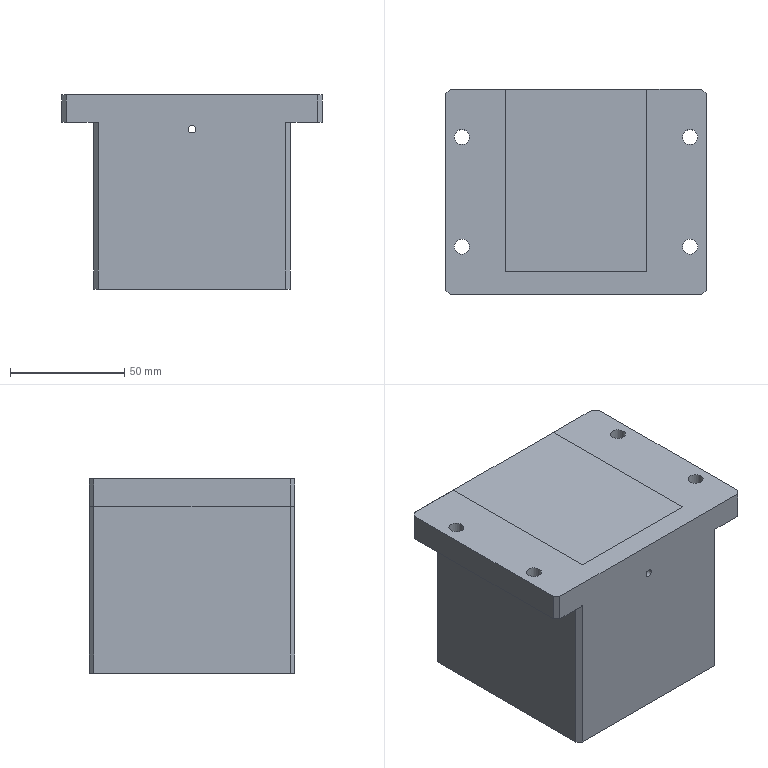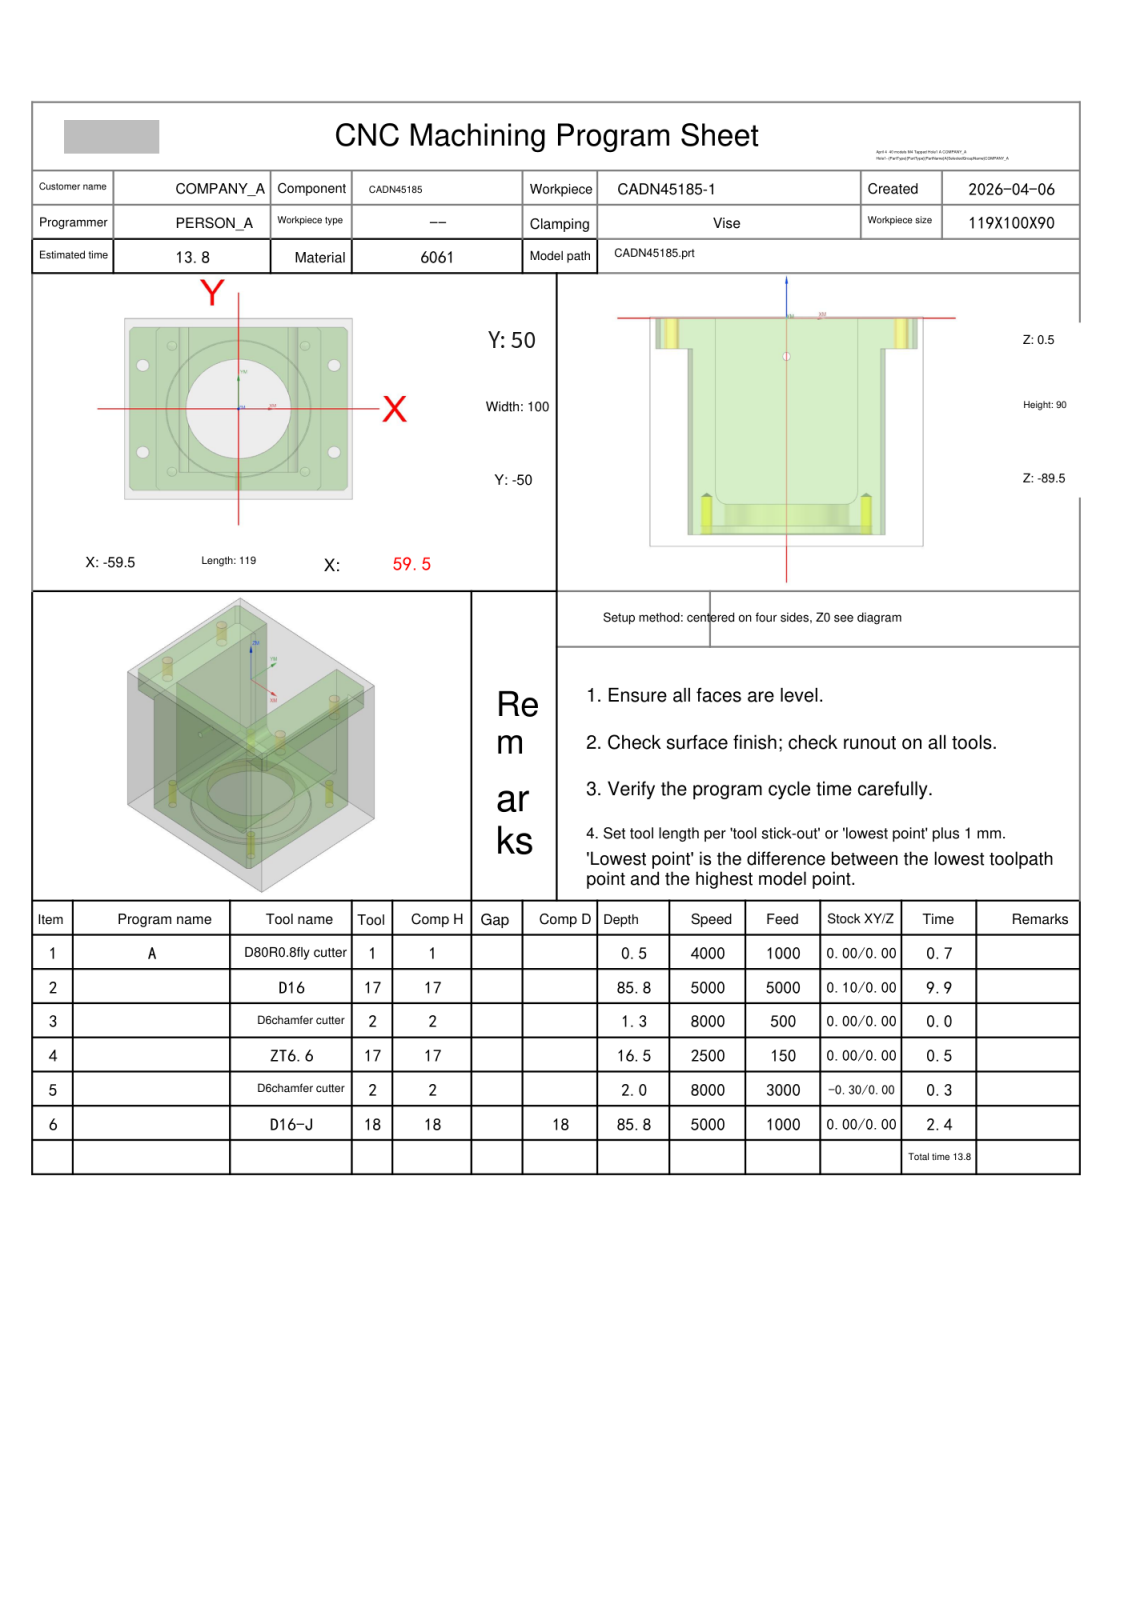NC program | NX | posted by the shop | part box 114 x 90 x 85 mm
Lines 1795 to 2085 of 2085:
N3 T02 M06
(D6chamfer cutter  D=6. R=0. H=02 ce=0.00 di=0.00)
G00 G90 G54 X50. Y-24. M03 S8000
G43 H02 Z20.
M08
G98 G81 X50. Y-24. Z-.8 R1. F500.
Y24.
X-50.
Y-24.
G80
G00 Z20.
G91 G28 Z0.0
M05
M09
G91 G28 Z0.0
M01
N4 T17 M06
(ZT6.6 D=6.6 DR_a=118 H=17)
G00 G90 G54 X50. Y-24. M03 S2500
G43 H17 Z20.
M08
G98 G83 X50. Y-24. Z-15.983 R1. F150. Q3.
Y24.
X-50.
Y-24.
G80
G00 Z20.
G91 G28 Z0.0
M05
M09
G91 G28 Z0.0
M01
N5 T02 M06
(D6chamfer cutter  D=6. R=0. H=02 ce=0.00 di=0.00)
G00 G90 G54 X.25 Y-47.128 M03 S8000
G43 H02 Z20.
M08
Z2.099
G01 Z-1.5 F3000.
G03 X.33 Y-46.828 I-.52 J.3
X.03 Y-46.308 I-.6 J0.0
G01 X0.0 Y-46.3
X-55.
X-55.254 Y-46.275
X-55.497 Y-46.201
X-55.722 Y-46.081
X-55.919 Y-45.919
X-57.919 Y-43.919
X-58.081 Y-43.722
X-58.201 Y-43.497
X-58.275 Y-43.254
X-58.3 Y-43.
Y43.
X-58.275 Y43.254
X-58.201 Y43.497
X-58.081 Y43.722
X-57.919 Y43.919
X-55.919 Y45.919
X-55.722 Y46.081
X-55.497 Y46.201
X-55.254 Y46.275
X-55. Y46.3
X55.
X55.254 Y46.275
X55.497 Y46.201
X55.722 Y46.081
X55.919 Y45.919
X57.919 Y43.919
X58.081 Y43.722
X58.201 Y43.498
X58.275 Y43.254
X58.3 Y43.
Y-43.
X58.275 Y-43.254
X58.201 Y-43.497
X58.081 Y-43.722
X57.919 Y-43.919
X55.919 Y-45.919
X55.722 Y-46.081
X55.497 Y-46.201
X55.254 Y-46.275
X55. Y-46.3
X0.0
X-.03 Y-46.308
G03 X-.33 Y-46.828 I.3 J-.52
X-.25 Y-47.128 I.6 J0.0
G01 Z2.099
G00 Z20.
G00 G90 X50.557 Y-25.5 M03 S8000
Z20.
Z-.5
G01 Z-1. F800.
X51.1
G03 X52.6 Y-24. I0.0 J1.5
X50. Y-21.4 I-2.6 J0.0
X47.4 Y-24. I0.0 J-2.6
X50. Y-26.6 I2.6 J0.0
X52.6 Y-24. I0.0 J2.6
X51.1 Y-22.5 I-1.5 J0.0
G01 X50.557
Z-.5
G00 Z20.
Y22.5
Z-.5
G01 Z-1.
X51.1
G03 X52.6 Y24. I0.0 J1.5
X50. Y26.6 I-2.6 J0.0
X47.4 Y24. I0.0 J-2.6
X50. Y21.4 I2.6 J0.0
X52.6 Y24. I0.0 J2.6
X51.1 Y25.5 I-1.5 J0.0
G01 X50.557
Z-.5
G00 Z20.
X-49.443 Y22.5
Z-.5
G01 Z-1.
X-48.9
G03 X-47.4 Y24. I0.0 J1.5
X-50. Y26.6 I-2.6 J0.0
X-52.6 Y24. I0.0 J-2.6
X-50. Y21.4 I2.6 J0.0
X-47.4 Y24. I0.0 J2.6
X-48.9 Y25.5 I-1.5 J0.0
G01 X-49.443
Z-.5
G00 Z20.
Y-25.5
Z-.5
G01 Z-1.
X-48.9
G03 X-47.4 Y-24. I0.0 J1.5
X-50. Y-21.4 I-2.6 J0.0
X-52.6 Y-24. I0.0 J-2.6
X-50. Y-26.6 I2.6 J0.0
X-47.4 Y-24. I0.0 J2.6
X-48.9 Y-22.5 I-1.5 J0.0
G01 X-49.443
Z-.5
G00 Z20.
G91 G28 Z0.0
M05
M09
G91 G28 Z0.0
M01
N6 T18 M06
(D16-J  D=16. R=0. H=18 ce=0.00 di=0.00)
G00 G90 G54 X-56.01 Y54.144 M03 S5000
G43 H18 Z20.
M08
Z-16.56
G01 Z-17.06 F1000.
G41 D18
X-55.998 Y53.944
G03 X-55. Y53. I.998 J.056
G01 X55.
G02 X60.657 Y50.657 I0.0 J-8.
G01 X62.657 Y48.657
G02 X65. Y43. I-5.657 J-5.657
G01 Y-43.
G02 X62.657 Y-48.657 I-8. J0.0
G01 X60.657 Y-50.657
G02 X55. Y-53. I-5.657 J5.657
G01 X-55.
G02 X-60.657 Y-50.657 I0.0 J8.
G01 X-62.657 Y-48.657
G02 X-65. Y-43. I5.657 J5.657
G01 Y43.
G02 X-62.657 Y48.657 I8. J0.0
G01 X-60.657 Y50.657
G02 X-55. Y53. I5.657 J-5.657
G01 X-54.5
G03 X-53.5 Y54. I0.0 J1.
G01 G40 Y54.2
Z-16.56
G00 Z20.
X-56.01 Y54.144
Z-33.62
G01 Z-34.12
G41 D18
X-55.998 Y53.944
G03 X-55. Y53. I.998 J.056
G01 X55.
G02 X60.657 Y50.657 I0.0 J-8.
G01 X62.657 Y48.657
G02 X65. Y43. I-5.657 J-5.657
G01 Y-43.
G02 X62.657 Y-48.657 I-8. J0.0
G01 X60.657 Y-50.657
G02 X55. Y-53. I-5.657 J5.657
G01 X-55.
G02 X-60.657 Y-50.657 I0.0 J8.
G01 X-62.657 Y-48.657
G02 X-65. Y-43. I5.657 J5.657
G01 Y43.
G02 X-62.657 Y48.657 I8. J0.0
G01 X-60.657 Y50.657
G02 X-55. Y53. I5.657 J-5.657
G01 X-54.5
G03 X-53.5 Y54. I0.0 J1.
G01 G40 Y54.2
Z-33.62
G00 Z20.
X-56.01 Y54.144
Z-50.68
G01 Z-51.18
G41 D18
X-55.998 Y53.944
G03 X-55. Y53. I.998 J.056
G01 X55.
G02 X60.657 Y50.657 I0.0 J-8.
G01 X62.657 Y48.657
G02 X65. Y43. I-5.657 J-5.657
G01 Y-43.
G02 X62.657 Y-48.657 I-8. J0.0
G01 X60.657 Y-50.657
G02 X55. Y-53. I-5.657 J5.657
G01 X-55.
G02 X-60.657 Y-50.657 I0.0 J8.
G01 X-62.657 Y-48.657
G02 X-65. Y-43. I5.657 J5.657
G01 Y43.
G02 X-62.657 Y48.657 I8. J0.0
G01 X-60.657 Y50.657
G02 X-55. Y53. I5.657 J-5.657
G01 X-54.5
G03 X-53.5 Y54. I0.0 J1.
G01 G40 Y54.2
Z-50.68
G00 Z20.
X-56.01 Y54.144
Z-67.74
G01 Z-68.24
G41 D18
X-55.998 Y53.944
G03 X-55. Y53. I.998 J.056
G01 X55.
G02 X60.657 Y50.657 I0.0 J-8.
G01 X62.657 Y48.657
G02 X65. Y43. I-5.657 J-5.657
G01 Y-43.
G02 X62.657 Y-48.657 I-8. J0.0
G01 X60.657 Y-50.657
G02 X55. Y-53. I-5.657 J5.657
G01 X-55.
G02 X-60.657 Y-50.657 I0.0 J8.
G01 X-62.657 Y-48.657
G02 X-65. Y-43. I5.657 J5.657
G01 Y43.
G02 X-62.657 Y48.657 I8. J0.0
G01 X-60.657 Y50.657
G02 X-55. Y53. I5.657 J-5.657
G01 X-54.5
G03 X-53.5 Y54. I0.0 J1.
G01 G40 Y54.2
Z-67.74
G00 Z20.
X-56.01 Y54.144
Z-84.8
G01 Z-85.3
G41 D18
X-55.998 Y53.944
G03 X-55. Y53. I.998 J.056
G01 X55.
G02 X60.657 Y50.657 I0.0 J-8.
G01 X62.657 Y48.657
G02 X65. Y43. I-5.657 J-5.657
G01 Y-43.
G02 X62.657 Y-48.657 I-8. J0.0
G01 X60.657 Y-50.657
G02 X55. Y-53. I-5.657 J5.657
G01 X-55.
G02 X-60.657 Y-50.657 I0.0 J8.
G01 X-62.657 Y-48.657
G02 X-65. Y-43. I5.657 J5.657
G01 Y43.
G02 X-62.657 Y48.657 I8. J0.0
G01 X-60.657 Y50.657
G02 X-55. Y53. I5.657 J-5.657
G01 X-54.5
G03 X-53.5 Y54. I0.0 J1.
G01 G40 Y54.2
Z-84.8
G00 Z20.
M05
M09
G91 G28 Z0.0
G91 G28 Y0.0
M30
%